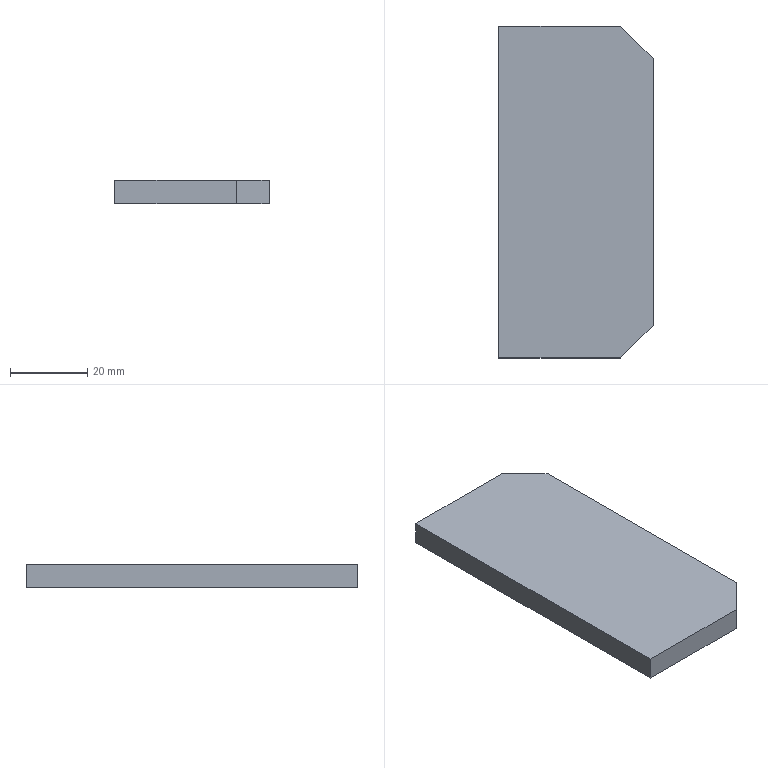Part | SolidWorks | features Chamfer 1, Extrusion 1 | 1 solid | 8 faces | box 40 x 86 x 6 mm | volume 20206 mm3 | plane 8
STEP:
#1=CARTESIAN_POINT('',(-20.,43.,0.));
#2=VERTEX_POINT('',#1);
#3=CARTESIAN_POINT('',(-20.,-43.,0.));
#4=VERTEX_POINT('',#3);
#5=CARTESIAN_POINT('',(-20.,43.,0.));
#6=DIRECTION('',(0.,-1.,0.));
#7=VECTOR('',#6,1000.);
#8=LINE('',#5,#7);
#9=EDGE_CURVE('',#2,#4,#8,.T.);
#10=ORIENTED_EDGE('',*,*,#9,.T.);
#11=CARTESIAN_POINT('',(-20.,-43.,6.));
#12=VERTEX_POINT('',#11);
#13=CARTESIAN_POINT('',(-20.,-43.,6.));
#14=DIRECTION('',(0.,0.,-1.));
#15=VECTOR('',#14,1000.);
#16=LINE('',#13,#15);
#17=EDGE_CURVE('',#12,#4,#16,.T.);
#18=ORIENTED_EDGE('',*,*,#17,.F.);
#19=CARTESIAN_POINT('',(-20.,43.,6.));
#20=VERTEX_POINT('',#19);
#21=CARTESIAN_POINT('',(-20.,43.,6.));
#22=DIRECTION('',(0.,-1.,0.));
#23=VECTOR('',#22,1000.);
#24=LINE('',#21,#23);
#25=EDGE_CURVE('',#20,#12,#24,.T.);
#26=ORIENTED_EDGE('',*,*,#25,.F.);
#27=CARTESIAN_POINT('',(-20.,43.,6.));
#28=DIRECTION('',(0.,0.,-1.));
#29=VECTOR('',#28,1000.);
#30=LINE('',#27,#29);
#31=EDGE_CURVE('',#20,#2,#30,.T.);
#32=ORIENTED_EDGE('',*,*,#31,.T.);
#33=EDGE_LOOP('',(#10,#18,#26,#32));
#34=FACE_OUTER_BOUND('',#33,.T.);
#35=CARTESIAN_POINT('',(-20.,43.,6.));
#36=DIRECTION('',(1.,0.,0.));
#37=DIRECTION('',(0.,1.,0.));
#38=AXIS2_PLACEMENT_3D('',#35,#36,#37);
#39=PLANE('',#38);
#40=ADVANCED_FACE('',(#34),#39,.F.);
#41=CARTESIAN_POINT('',(11.5,-43.,0.));
#42=VERTEX_POINT('',#41);
#43=CARTESIAN_POINT('',(20.,-43.,0.));
#44=DIRECTION('',(1.,0.,0.));
#45=VECTOR('',#44,1000.);
#46=LINE('',#43,#45);
#47=EDGE_CURVE('',#4,#42,#46,.T.);
#48=ORIENTED_EDGE('',*,*,#47,.T.);
#49=CARTESIAN_POINT('',(11.5,-43.,6.));
#50=VERTEX_POINT('',#49);
#51=CARTESIAN_POINT('',(11.5,-43.,6.));
#52=DIRECTION('',(0.,0.,1.));
#53=VECTOR('',#52,1000.);
#54=LINE('',#51,#53);
#55=EDGE_CURVE('',#42,#50,#54,.T.);
#56=ORIENTED_EDGE('',*,*,#55,.T.);
#57=CARTESIAN_POINT('',(20.,-43.,6.));
#58=DIRECTION('',(1.,0.,0.));
#59=VECTOR('',#58,1000.);
#60=LINE('',#57,#59);
#61=EDGE_CURVE('',#12,#50,#60,.T.);
#62=ORIENTED_EDGE('',*,*,#61,.F.);
#63=ORIENTED_EDGE('',*,*,#17,.T.);
#64=EDGE_LOOP('',(#48,#56,#62,#63));
#65=FACE_OUTER_BOUND('',#64,.T.);
#66=CARTESIAN_POINT('',(20.,-43.,6.));
#67=DIRECTION('',(0.,1.,0.));
#68=DIRECTION('',(-1.,0.,0.));
#69=AXIS2_PLACEMENT_3D('',#66,#67,#68);
#70=PLANE('',#69);
#71=ADVANCED_FACE('',(#65),#70,.F.);
#72=CARTESIAN_POINT('',(20.,-34.5,6.));
#73=VERTEX_POINT('',#72);
#74=CARTESIAN_POINT('',(20.,34.5,6.));
#75=VERTEX_POINT('',#74);
#76=CARTESIAN_POINT('',(20.,43.,6.));
#77=DIRECTION('',(0.,1.,0.));
#78=VECTOR('',#77,1000.);
#79=LINE('',#76,#78);
#80=EDGE_CURVE('',#73,#75,#79,.T.);
#81=ORIENTED_EDGE('',*,*,#80,.F.);
#82=CARTESIAN_POINT('',(20.,-34.5,0.));
#83=VERTEX_POINT('',#82);
#84=CARTESIAN_POINT('',(20.,-34.5,6.));
#85=DIRECTION('',(0.,0.,-1.));
#86=VECTOR('',#85,1000.);
#87=LINE('',#84,#86);
#88=EDGE_CURVE('',#73,#83,#87,.T.);
#89=ORIENTED_EDGE('',*,*,#88,.T.);
#90=CARTESIAN_POINT('',(20.,34.5,0.));
#91=VERTEX_POINT('',#90);
#92=CARTESIAN_POINT('',(20.,43.,0.));
#93=DIRECTION('',(0.,1.,0.));
#94=VECTOR('',#93,1000.);
#95=LINE('',#92,#94);
#96=EDGE_CURVE('',#83,#91,#95,.T.);
#97=ORIENTED_EDGE('',*,*,#96,.T.);
#98=CARTESIAN_POINT('',(20.,34.5,6.));
#99=DIRECTION('',(0.,0.,1.));
#100=VECTOR('',#99,1000.);
#101=LINE('',#98,#100);
#102=EDGE_CURVE('',#91,#75,#101,.T.);
#103=ORIENTED_EDGE('',*,*,#102,.T.);
#104=EDGE_LOOP('',(#81,#89,#97,#103));
#105=FACE_OUTER_BOUND('',#104,.T.);
#106=CARTESIAN_POINT('',(20.,43.,6.));
#107=DIRECTION('',(-1.,0.,0.));
#108=DIRECTION('',(0.,-1.,0.));
#109=AXIS2_PLACEMENT_3D('',#106,#107,#108);
#110=PLANE('',#109);
#111=ADVANCED_FACE('',(#105),#110,.F.);
#112=CARTESIAN_POINT('',(11.5,43.,6.));
#113=VERTEX_POINT('',#112);
#114=CARTESIAN_POINT('',(20.,43.,6.));
#115=DIRECTION('',(-1.,0.,0.));
#116=VECTOR('',#115,1000.);
#117=LINE('',#114,#116);
#118=EDGE_CURVE('',#113,#20,#117,.T.);
#119=ORIENTED_EDGE('',*,*,#118,.F.);
#120=CARTESIAN_POINT('',(11.5,43.,0.));
#121=VERTEX_POINT('',#120);
#122=CARTESIAN_POINT('',(11.5,43.,6.));
#123=DIRECTION('',(0.,0.,-1.));
#124=VECTOR('',#123,1000.);
#125=LINE('',#122,#124);
#126=EDGE_CURVE('',#113,#121,#125,.T.);
#127=ORIENTED_EDGE('',*,*,#126,.T.);
#128=CARTESIAN_POINT('',(20.,43.,0.));
#129=DIRECTION('',(-1.,0.,0.));
#130=VECTOR('',#129,1000.);
#131=LINE('',#128,#130);
#132=EDGE_CURVE('',#121,#2,#131,.T.);
#133=ORIENTED_EDGE('',*,*,#132,.T.);
#134=ORIENTED_EDGE('',*,*,#31,.F.);
#135=EDGE_LOOP('',(#119,#127,#133,#134));
#136=FACE_OUTER_BOUND('',#135,.T.);
#137=CARTESIAN_POINT('',(20.,43.,6.));
#138=DIRECTION('',(0.,-1.,0.));
#139=DIRECTION('',(0.,0.,-1.));
#140=AXIS2_PLACEMENT_3D('',#137,#138,#139);
#141=PLANE('',#140);
#142=ADVANCED_FACE('',(#136),#141,.F.);
#143=ORIENTED_EDGE('',*,*,#61,.T.);
#144=CARTESIAN_POINT('',(20.,-34.5,6.));
#145=DIRECTION('',(0.7071,0.7071,0.));
#146=VECTOR('',#145,1000.);
#147=LINE('',#144,#146);
#148=EDGE_CURVE('',#50,#73,#147,.T.);
#149=ORIENTED_EDGE('',*,*,#148,.T.);
#150=ORIENTED_EDGE('',*,*,#80,.T.);
#151=CARTESIAN_POINT('',(11.5,43.,6.));
#152=DIRECTION('',(-0.7071,0.7071,0.));
#153=VECTOR('',#152,1000.);
#154=LINE('',#151,#153);
#155=EDGE_CURVE('',#75,#113,#154,.T.);
#156=ORIENTED_EDGE('',*,*,#155,.T.);
#157=ORIENTED_EDGE('',*,*,#118,.T.);
#158=ORIENTED_EDGE('',*,*,#25,.T.);
#159=EDGE_LOOP('',(#143,#149,#150,#156,#157,#158));
#160=FACE_OUTER_BOUND('',#159,.T.);
#161=CARTESIAN_POINT('',(0.,0.,6.));
#162=DIRECTION('',(0.,0.,-1.));
#163=DIRECTION('',(-1.,0.,0.));
#164=AXIS2_PLACEMENT_3D('',#161,#162,#163);
#165=PLANE('',#164);
#166=ADVANCED_FACE('',(#160),#165,.F.);
#167=ORIENTED_EDGE('',*,*,#96,.F.);
#168=CARTESIAN_POINT('',(27.25,-27.25,0.));
#169=DIRECTION('',(-0.7071,-0.7071,0.));
#170=VECTOR('',#169,1000.);
#171=LINE('',#168,#170);
#172=EDGE_CURVE('',#83,#42,#171,.T.);
#173=ORIENTED_EDGE('',*,*,#172,.T.);
#174=ORIENTED_EDGE('',*,*,#47,.F.);
#175=ORIENTED_EDGE('',*,*,#9,.F.);
#176=ORIENTED_EDGE('',*,*,#132,.F.);
#177=CARTESIAN_POINT('',(27.25,27.25,0.));
#178=DIRECTION('',(0.7071,-0.7071,0.));
#179=VECTOR('',#178,1000.);
#180=LINE('',#177,#179);
#181=EDGE_CURVE('',#121,#91,#180,.T.);
#182=ORIENTED_EDGE('',*,*,#181,.T.);
#183=EDGE_LOOP('',(#167,#173,#174,#175,#176,#182));
#184=FACE_OUTER_BOUND('',#183,.T.);
#185=CARTESIAN_POINT('',(0.,0.,0.));
#186=DIRECTION('',(0.,0.,-1.));
#187=DIRECTION('',(-1.,0.,0.));
#188=AXIS2_PLACEMENT_3D('',#185,#186,#187);
#189=PLANE('',#188);
#190=ADVANCED_FACE('',(#184),#189,.T.);
#191=ORIENTED_EDGE('',*,*,#148,.F.);
#192=ORIENTED_EDGE('',*,*,#55,.F.);
#193=ORIENTED_EDGE('',*,*,#172,.F.);
#194=ORIENTED_EDGE('',*,*,#88,.F.);
#195=EDGE_LOOP('',(#191,#192,#193,#194));
#196=FACE_OUTER_BOUND('',#195,.T.);
#197=CARTESIAN_POINT('',(20.,-34.5,6.));
#198=DIRECTION('',(-0.7071,0.7071,0.));
#199=DIRECTION('',(0.,0.,-1.));
#200=AXIS2_PLACEMENT_3D('',#197,#198,#199);
#201=PLANE('',#200);
#202=ADVANCED_FACE('',(#196),#201,.F.);
#203=ORIENTED_EDGE('',*,*,#155,.F.);
#204=ORIENTED_EDGE('',*,*,#102,.F.);
#205=ORIENTED_EDGE('',*,*,#181,.F.);
#206=ORIENTED_EDGE('',*,*,#126,.F.);
#207=EDGE_LOOP('',(#203,#204,#205,#206));
#208=FACE_OUTER_BOUND('',#207,.T.);
#209=CARTESIAN_POINT('',(11.5,43.,6.));
#210=DIRECTION('',(-0.7071,-0.7071,0.));
#211=DIRECTION('',(0.,0.,-1.));
#212=AXIS2_PLACEMENT_3D('',#209,#210,#211);
#213=PLANE('',#212);
#214=ADVANCED_FACE('',(#208),#213,.F.);
#215=CLOSED_SHELL('',(#40,#71,#111,#142,#166,#190,#202,#214));
#216=MANIFOLD_SOLID_BREP('',#215);
#217=CARTESIAN_POINT('',(0.,0.,0.));
#218=DIRECTION('',(0.,0.,1.));
#219=DIRECTION('',(1.,0.,0.));
#220=AXIS2_PLACEMENT_3D('',#217,#218,#219);
#221=(LENGTH_UNIT()NAMED_UNIT(*)SI_UNIT(.MILLI.,.METRE.));
#222=UNCERTAINTY_MEASURE_WITH_UNIT(LENGTH_MEASURE(0.00001),#221,'','');
#223=(NAMED_UNIT(*)PLANE_ANGLE_UNIT()SI_UNIT($,.RADIAN.));
#224=(NAMED_UNIT(*)SI_UNIT($,.STERADIAN.)SOLID_ANGLE_UNIT());
#225=(GEOMETRIC_REPRESENTATION_CONTEXT(3)GLOBAL_UNCERTAINTY_ASSIGNED_CONTEXT((#222))GLOBAL_UNIT_ASSIGNED_CONTEXT((#221,#223,#224))REPRESENTATION_CONTEXT('',''));
#226=ADVANCED_BREP_SHAPE_REPRESENTATION('',(#216,#220),#225);